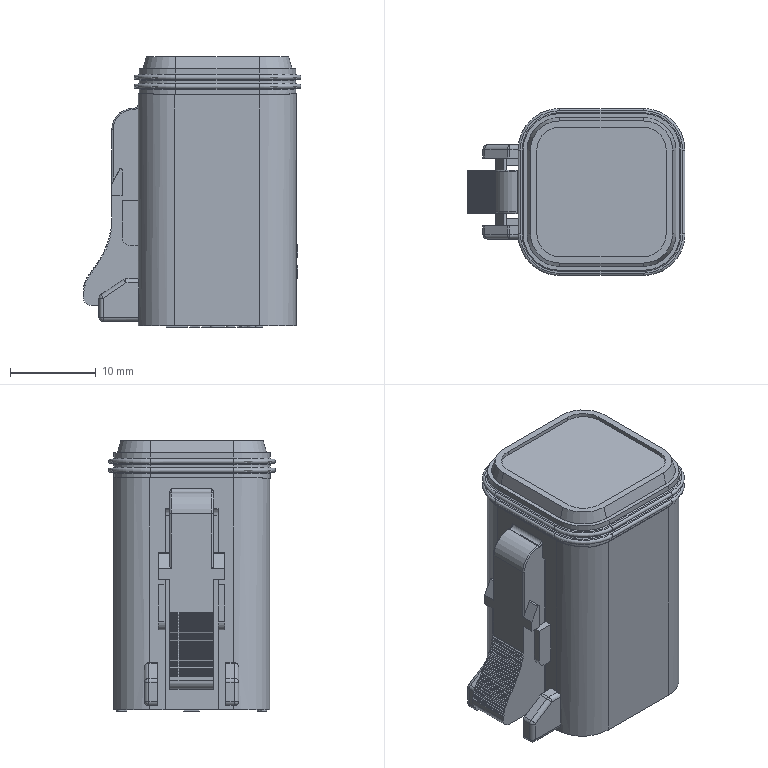Part | NX | features BREP 1 | 1 solid | 1052 faces | box 25.459 x 19.5 x 31.65 mm | volume 10405 mm3 | plane 883 | cylinder 107 | torus 40 | cone 16 | sphere 6 | commonest cylinder face diameters 0.2 x24 0.24 x16 8.5 x16 1 x15 1.2 x12 0.52 x8